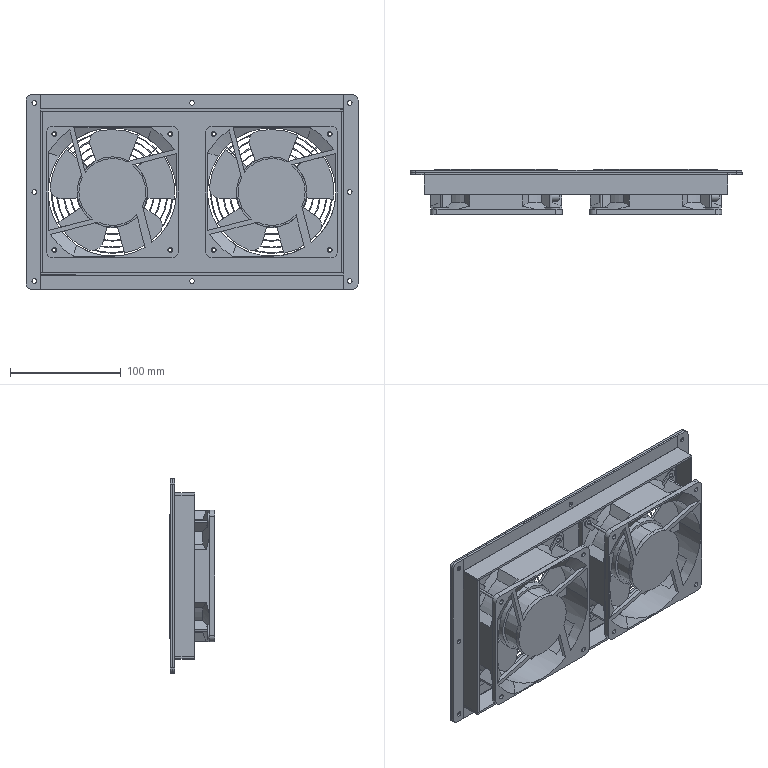Part | SolidWorks | 9 solids | 944 faces | box 300 x 40.8 x 176 mm | volume 500898 mm3 | cylinder 458 | plane 432 | cone 54 | commonest cylinder face diameters 4.293 x32 9.53 x24 4.2 x20 5.3 x18 6.7 x18 3.3 x16